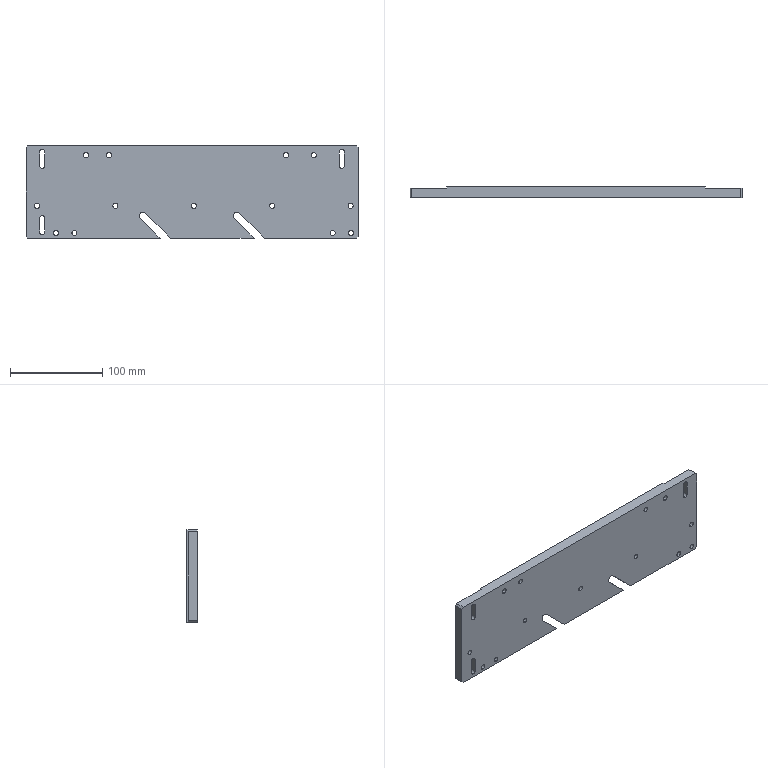Part | SolidWorks | features ICE 12, Cut 3, Chamfer 1, Extrusion 1, LPattern 1 | 1 solid | 109 faces | box 360 x 11.8 x 100 mm | volume 390446 mm3 | cylinder 62 | plane 47 | commonest cylinder face diameters 5.5 x35 12 x15 10 x10 8 x2